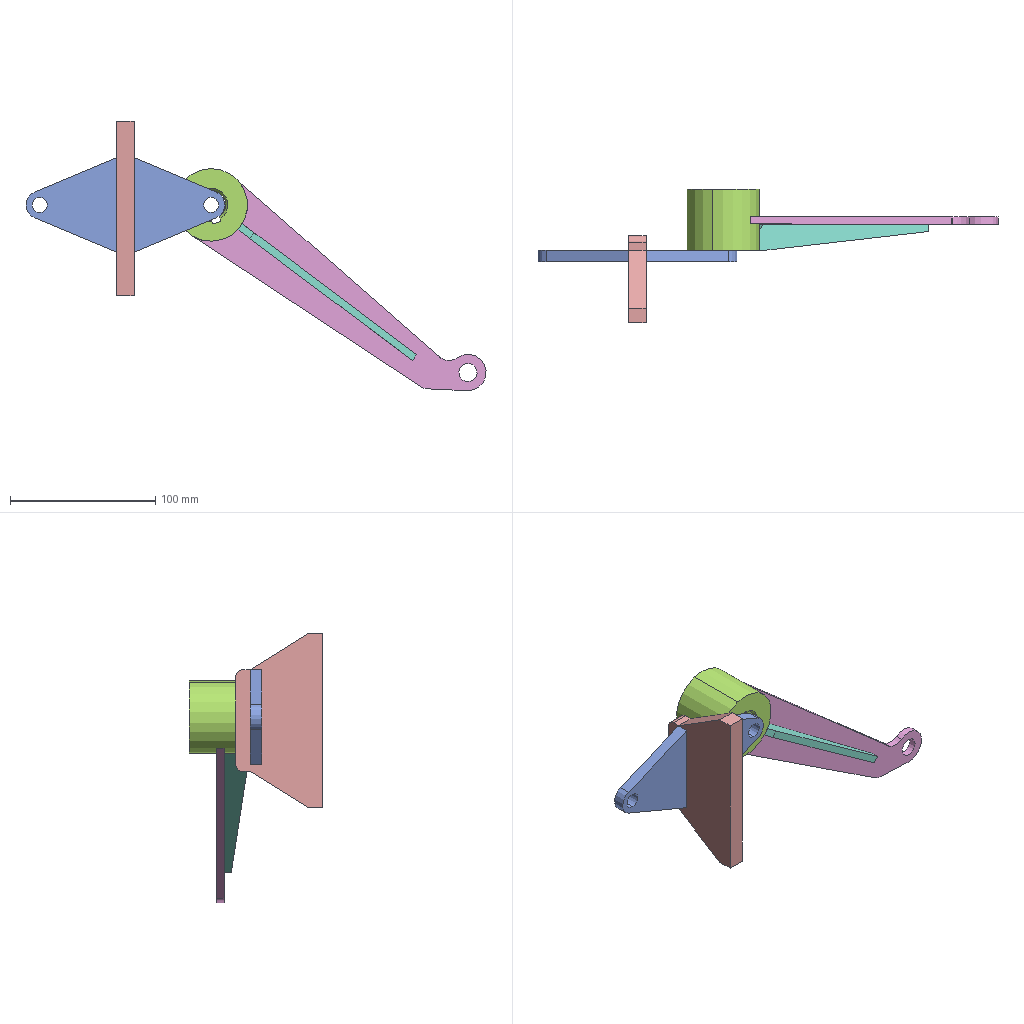Assembly | SolidWorks | 5 different items | 6 placed | box 316 x 92 x 185 mm
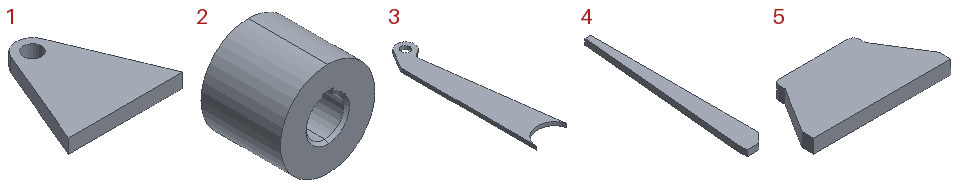Parts list (item | quantity | size | volume | features):
1 | x2 | 65 x 62.5 x 8 mm | 18605 mm3 | features Extrusion 1
2 | x1 | 50 x 42 x 50 mm | 68393 mm3 | features Chamfer 1, Extrusion 1
3 | x1 | 48.98 x 222.5 x 5 mm | 33616 mm3 | features Extrusion 1
4 | x1 | 18 x 150 x 5 mm | 8790 mm3 | features Extrusion 1
5 | x1 | 120 x 60 x 12 mm | 68271 mm3 | features Extrusion 1, Fillet 1
Mates (type | each side: item.copy, entity, surface, feature):
Coincident | 5.1 face plane Boss-Extrude1 | 1.1 face plane Boss-Extrude1
DistanceDim | 5.1 face plane Boss-Extrude1 | 1.1 face plane Boss-Extrude1
Coincident | 5.1 face plane Boss-Extrude1 | 1.2 face plane Boss-Extrude1
Coincident | 1.1 face plane Boss-Extrude1 | 1.2 face plane Boss-Extrude1
Concentric | 2.1 face cylinder Boss-Extrude1 | 3.1 face cylinder Boss-Extrude1
DistanceDim | 3.1 face plane Boss-Extrude1 | 2.1 face plane Boss-Extrude1
Width | 4.1 face plane Boss-Extrude1 | 4.1 face plane Boss-Extrude1 | 2.1 face cylinder Boss-Extrude1
Tangent | 2.1 face cylinder Boss-Extrude1 | 4.1 face plane Boss-Extrude1
Coincident | 3.1 face plane Boss-Extrude1 | 4.1 face plane Boss-Extrude1
PlanarAngleDim | 3.1 face plane Boss-Extrude1 | 4.1 face plane Boss-Extrude1
Concentric | 1.2 face cylinder Boss-Extrude1 | 2.1 face cylinder Boss-Extrude1
Coincident | 1.2 face plane Boss-Extrude1 | 2.1 face plane Boss-Extrude1
Coincident | 1.1 plane | 1.2 plane
Coincident | 5.1 face plane Boss-Extrude1 | 1.1 edge